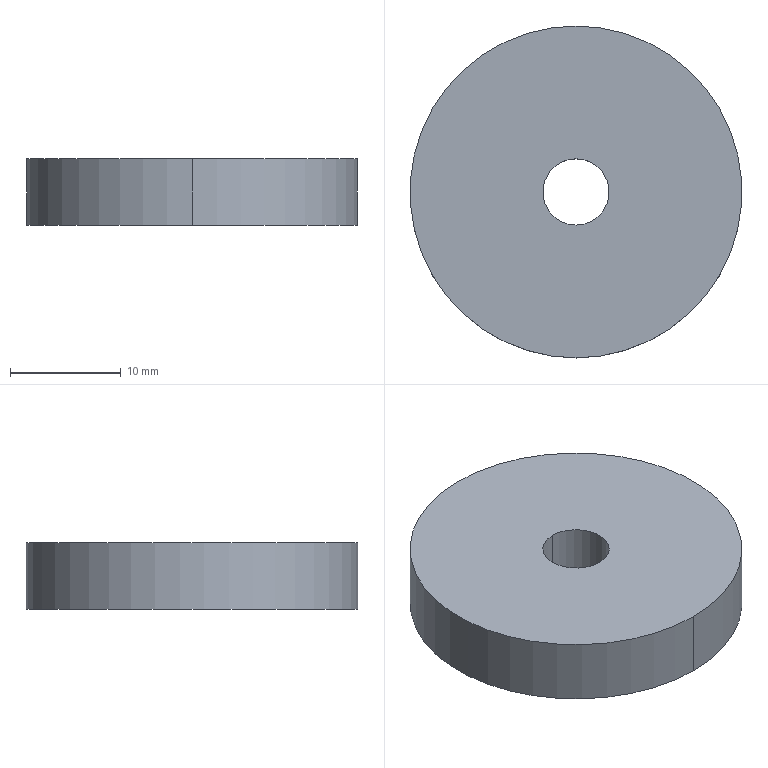Part | SolidWorks | features BaseBody 1 | 1 solid | 6 faces | box 30 x 30 x 6 mm | volume 4072 mm3 | cylinder 4 | plane 2 | commonest cylinder face diameters 6 x2 30 x2
STEP:
#1=CARTESIAN_POINT('',(591.519,-172.648,7.889));
#2=VERTEX_POINT('',#1);
#3=CARTESIAN_POINT('',(591.519,-202.648,7.889));
#4=VERTEX_POINT('',#3);
#5=CARTESIAN_POINT('',(591.519,-187.648,7.889));
#6=DIRECTION('',(-0.000000001,0.000000003,-1.));
#7=DIRECTION('',(0.,1.,0.000000003));
#8=AXIS2_PLACEMENT_3D('',#5,#6,#7);
#9=CIRCLE('',#8,15.);
#10=EDGE_CURVE('',#2,#4,#9,.T.);
#11=ORIENTED_EDGE('',*,*,#10,.T.);
#12=CARTESIAN_POINT('',(591.519,-202.648,1.889));
#13=VERTEX_POINT('',#12);
#14=CARTESIAN_POINT('',(591.519,-202.648,1.889));
#15=DIRECTION('',(-0.000000001,0.000000003,-1.));
#16=VECTOR('',#15,1000.);
#17=LINE('',#14,#16);
#18=EDGE_CURVE('',#4,#13,#17,.T.);
#19=ORIENTED_EDGE('',*,*,#18,.T.);
#20=CARTESIAN_POINT('',(591.519,-172.648,1.889));
#21=VERTEX_POINT('',#20);
#22=CARTESIAN_POINT('',(591.519,-187.648,1.889));
#23=DIRECTION('',(0.000000001,-0.000000003,1.));
#24=DIRECTION('',(0.,1.,0.000000003));
#25=AXIS2_PLACEMENT_3D('',#22,#23,#24);
#26=CIRCLE('',#25,15.);
#27=EDGE_CURVE('',#13,#21,#26,.T.);
#28=ORIENTED_EDGE('',*,*,#27,.T.);
#29=CARTESIAN_POINT('',(591.519,-172.648,1.889));
#30=DIRECTION('',(-0.000000001,0.000000003,-1.));
#31=VECTOR('',#30,1000.);
#32=LINE('',#29,#31);
#33=EDGE_CURVE('',#2,#21,#32,.T.);
#34=ORIENTED_EDGE('',*,*,#33,.F.);
#35=EDGE_LOOP('',(#11,#19,#28,#34));
#36=FACE_OUTER_BOUND('',#35,.T.);
#37=CARTESIAN_POINT('',(591.519,-187.648,1.889));
#38=DIRECTION('',(-0.000000001,0.000000003,-1.));
#39=DIRECTION('',(0.,1.,0.000000003));
#40=AXIS2_PLACEMENT_3D('',#37,#38,#39);
#41=CYLINDRICAL_SURFACE('',#40,15.);
#42=ADVANCED_FACE('',(#36),#41,.T.);
#43=CARTESIAN_POINT('',(591.519,-190.648,1.889));
#44=VERTEX_POINT('',#43);
#45=CARTESIAN_POINT('',(591.519,-184.648,1.889));
#46=VERTEX_POINT('',#45);
#47=CARTESIAN_POINT('',(591.519,-187.648,1.889));
#48=DIRECTION('',(-0.000000001,0.000000003,-1.));
#49=DIRECTION('',(0.,-1.,-0.000000003));
#50=AXIS2_PLACEMENT_3D('',#47,#48,#49);
#51=CIRCLE('',#50,3.);
#52=EDGE_CURVE('',#44,#46,#51,.T.);
#53=ORIENTED_EDGE('',*,*,#52,.T.);
#54=CARTESIAN_POINT('',(591.519,-184.648,7.889));
#55=VERTEX_POINT('',#54);
#56=CARTESIAN_POINT('',(591.519,-184.648,7.889));
#57=DIRECTION('',(0.000000001,-0.000000003,1.));
#58=VECTOR('',#57,1000.);
#59=LINE('',#56,#58);
#60=EDGE_CURVE('',#46,#55,#59,.T.);
#61=ORIENTED_EDGE('',*,*,#60,.T.);
#62=CARTESIAN_POINT('',(591.519,-190.648,7.889));
#63=VERTEX_POINT('',#62);
#64=CARTESIAN_POINT('',(591.519,-187.648,7.889));
#65=DIRECTION('',(-0.000000001,0.000000003,-1.));
#66=DIRECTION('',(0.,-1.,-0.000000003));
#67=AXIS2_PLACEMENT_3D('',#64,#65,#66);
#68=CIRCLE('',#67,3.);
#69=EDGE_CURVE('',#63,#55,#68,.T.);
#70=ORIENTED_EDGE('',*,*,#69,.F.);
#71=CARTESIAN_POINT('',(591.519,-190.648,7.889));
#72=DIRECTION('',(0.000000001,-0.000000003,1.));
#73=VECTOR('',#72,1000.);
#74=LINE('',#71,#73);
#75=EDGE_CURVE('',#44,#63,#74,.T.);
#76=ORIENTED_EDGE('',*,*,#75,.F.);
#77=EDGE_LOOP('',(#53,#61,#70,#76));
#78=FACE_OUTER_BOUND('',#77,.T.);
#79=CARTESIAN_POINT('',(591.519,-187.648,7.889));
#80=DIRECTION('',(0.000000001,-0.000000003,1.));
#81=DIRECTION('',(0.,-1.,-0.000000003));
#82=AXIS2_PLACEMENT_3D('',#79,#80,#81);
#83=CYLINDRICAL_SURFACE('',#82,3.);
#84=ADVANCED_FACE('',(#78),#83,.F.);
#85=CARTESIAN_POINT('',(591.519,-187.648,1.889));
#86=DIRECTION('',(0.000000001,-0.000000003,1.));
#87=DIRECTION('',(0.,1.,0.000000003));
#88=AXIS2_PLACEMENT_3D('',#85,#86,#87);
#89=CIRCLE('',#88,15.);
#90=EDGE_CURVE('',#21,#13,#89,.T.);
#91=ORIENTED_EDGE('',*,*,#90,.F.);
#92=ORIENTED_EDGE('',*,*,#27,.F.);
#93=EDGE_LOOP('',(#91,#92));
#94=FACE_OUTER_BOUND('',#93,.T.);
#95=ORIENTED_EDGE('',*,*,#52,.F.);
#96=CARTESIAN_POINT('',(591.519,-187.648,1.889));
#97=DIRECTION('',(-0.000000001,0.000000003,-1.));
#98=DIRECTION('',(0.,-1.,-0.000000003));
#99=AXIS2_PLACEMENT_3D('',#96,#97,#98);
#100=CIRCLE('',#99,3.);
#101=EDGE_CURVE('',#46,#44,#100,.T.);
#102=ORIENTED_EDGE('',*,*,#101,.F.);
#103=EDGE_LOOP('',(#95,#102));
#104=FACE_BOUND('',#103,.T.);
#105=CARTESIAN_POINT('',(591.519,-187.648,1.889));
#106=DIRECTION('',(0.000000001,-0.000000003,1.));
#107=DIRECTION('',(0.,-1.,-0.000000003));
#108=AXIS2_PLACEMENT_3D('',#105,#106,#107);
#109=PLANE('',#108);
#110=ADVANCED_FACE('',(#94,#104),#109,.F.);
#111=ORIENTED_EDGE('',*,*,#18,.F.);
#112=CARTESIAN_POINT('',(591.519,-187.648,7.889));
#113=DIRECTION('',(-0.000000001,0.000000003,-1.));
#114=DIRECTION('',(0.,1.,0.000000003));
#115=AXIS2_PLACEMENT_3D('',#112,#113,#114);
#116=CIRCLE('',#115,15.);
#117=EDGE_CURVE('',#4,#2,#116,.T.);
#118=ORIENTED_EDGE('',*,*,#117,.T.);
#119=ORIENTED_EDGE('',*,*,#33,.T.);
#120=ORIENTED_EDGE('',*,*,#90,.T.);
#121=EDGE_LOOP('',(#111,#118,#119,#120));
#122=FACE_OUTER_BOUND('',#121,.T.);
#123=CARTESIAN_POINT('',(591.519,-187.648,1.889));
#124=DIRECTION('',(-0.000000001,0.000000003,-1.));
#125=DIRECTION('',(0.,1.,0.000000003));
#126=AXIS2_PLACEMENT_3D('',#123,#124,#125);
#127=CYLINDRICAL_SURFACE('',#126,15.);
#128=ADVANCED_FACE('',(#122),#127,.T.);
#129=ORIENTED_EDGE('',*,*,#60,.F.);
#130=ORIENTED_EDGE('',*,*,#101,.T.);
#131=ORIENTED_EDGE('',*,*,#75,.T.);
#132=CARTESIAN_POINT('',(591.519,-187.648,7.889));
#133=DIRECTION('',(-0.000000001,0.000000003,-1.));
#134=DIRECTION('',(0.,-1.,-0.000000003));
#135=AXIS2_PLACEMENT_3D('',#132,#133,#134);
#136=CIRCLE('',#135,3.);
#137=EDGE_CURVE('',#55,#63,#136,.T.);
#138=ORIENTED_EDGE('',*,*,#137,.F.);
#139=EDGE_LOOP('',(#129,#130,#131,#138));
#140=FACE_OUTER_BOUND('',#139,.T.);
#141=CARTESIAN_POINT('',(591.519,-187.648,7.889));
#142=DIRECTION('',(0.000000001,-0.000000003,1.));
#143=DIRECTION('',(0.,-1.,-0.000000003));
#144=AXIS2_PLACEMENT_3D('',#141,#142,#143);
#145=CYLINDRICAL_SURFACE('',#144,3.);
#146=ADVANCED_FACE('',(#140),#145,.F.);
#147=ORIENTED_EDGE('',*,*,#10,.F.);
#148=ORIENTED_EDGE('',*,*,#117,.F.);
#149=EDGE_LOOP('',(#147,#148));
#150=FACE_OUTER_BOUND('',#149,.T.);
#151=ORIENTED_EDGE('',*,*,#69,.T.);
#152=ORIENTED_EDGE('',*,*,#137,.T.);
#153=EDGE_LOOP('',(#151,#152));
#154=FACE_BOUND('',#153,.T.);
#155=CARTESIAN_POINT('',(591.519,-187.648,7.889));
#156=DIRECTION('',(0.000000001,-0.000000003,1.));
#157=DIRECTION('',(0.,-1.,-0.000000003));
#158=AXIS2_PLACEMENT_3D('',#155,#156,#157);
#159=PLANE('',#158);
#160=ADVANCED_FACE('',(#150,#154),#159,.T.);
#161=CLOSED_SHELL('',(#42,#84,#110,#128,#146,#160));
#162=MANIFOLD_SOLID_BREP('',#161);
#163=CARTESIAN_POINT('',(0.,0.,0.));
#164=DIRECTION('',(0.,0.,1.));
#165=DIRECTION('',(1.,0.,0.));
#166=AXIS2_PLACEMENT_3D('',#163,#164,#165);
#167=(LENGTH_UNIT()NAMED_UNIT(*)SI_UNIT(.MILLI.,.METRE.));
#168=UNCERTAINTY_MEASURE_WITH_UNIT(LENGTH_MEASURE(0.00001),#167,'','');
#169=(NAMED_UNIT(*)PLANE_ANGLE_UNIT()SI_UNIT($,.RADIAN.));
#170=(NAMED_UNIT(*)SI_UNIT($,.STERADIAN.)SOLID_ANGLE_UNIT());
#171=(GEOMETRIC_REPRESENTATION_CONTEXT(3)GLOBAL_UNCERTAINTY_ASSIGNED_CONTEXT((#168))GLOBAL_UNIT_ASSIGNED_CONTEXT((#167,#169,#170))REPRESENTATION_CONTEXT('',''));
#172=ADVANCED_BREP_SHAPE_REPRESENTATION('',(#162,#166),#171);